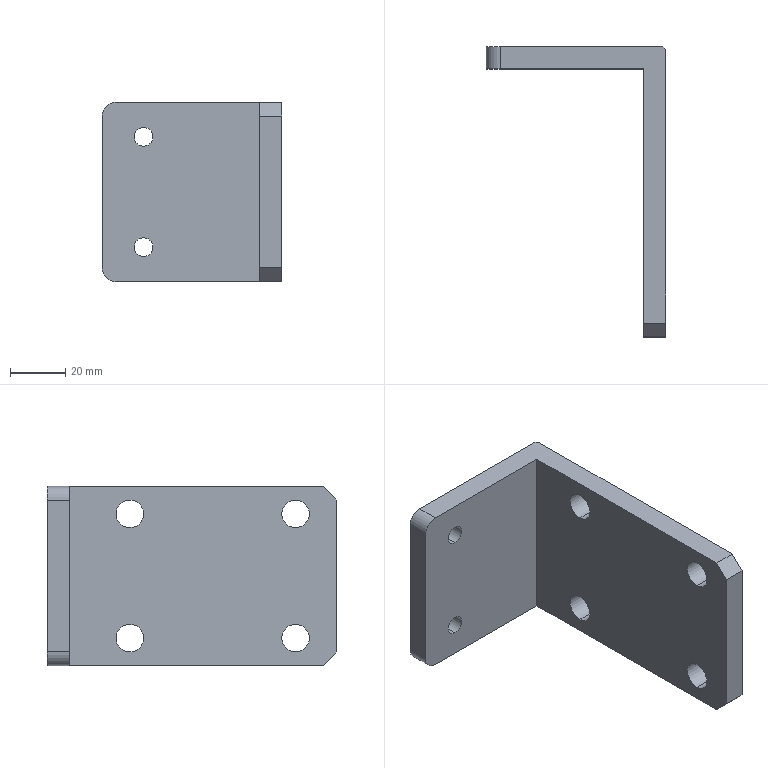Part | NX | features BREP 1 | 1 solid | 25 faces | box 65 x 105 x 65 mm | volume 80827 mm3 | cylinder 14 | plane 11 | commonest cylinder face diameters 10 x10 6.8 x4
STEP:
#1=CARTESIAN_POINT('',(0.,-30.,5.));
#2=VERTEX_POINT('',#1);
#3=CARTESIAN_POINT('',(0.,-30.,15.));
#4=VERTEX_POINT('',#3);
#5=CARTESIAN_POINT('',(0.,-30.,10.));
#6=DIRECTION('',(-1.,0.,0.));
#7=DIRECTION('',(0.,0.,1.));
#8=AXIS2_PLACEMENT_3D('',#5,#6,#7);
#9=CIRCLE('',#8,5.);
#10=EDGE_CURVE('',#2,#4,#9,.T.);
#11=ORIENTED_EDGE('',*,*,#10,.F.);
#12=CARTESIAN_POINT('',(-8.,-30.,5.));
#13=VERTEX_POINT('',#12);
#14=CARTESIAN_POINT('',(-8.,-30.,5.));
#15=DIRECTION('',(-1.,0.,0.));
#16=VECTOR('',#15,1000.);
#17=LINE('',#14,#16);
#18=EDGE_CURVE('',#13,#2,#17,.F.);
#19=ORIENTED_EDGE('',*,*,#18,.F.);
#20=CARTESIAN_POINT('',(-8.,-30.,15.));
#21=VERTEX_POINT('',#20);
#22=CARTESIAN_POINT('',(-8.,-30.,10.));
#23=DIRECTION('',(-1.,0.,0.));
#24=DIRECTION('',(0.,0.,1.));
#25=AXIS2_PLACEMENT_3D('',#22,#23,#24);
#26=CIRCLE('',#25,5.);
#27=EDGE_CURVE('',#13,#21,#26,.T.);
#28=ORIENTED_EDGE('',*,*,#27,.T.);
#29=CARTESIAN_POINT('',(-8.,-30.,15.));
#30=DIRECTION('',(-1.,0.,0.));
#31=VECTOR('',#30,1000.);
#32=LINE('',#29,#31);
#33=EDGE_CURVE('',#21,#4,#32,.F.);
#34=ORIENTED_EDGE('',*,*,#33,.T.);
#35=EDGE_LOOP('',(#11,#19,#28,#34));
#36=FACE_BOUND('',#35,.T.);
#37=CARTESIAN_POINT('',(-8.,-30.,10.));
#38=DIRECTION('',(-1.,0.,0.));
#39=DIRECTION('',(0.,0.,1.));
#40=AXIS2_PLACEMENT_3D('',#37,#38,#39);
#41=CYLINDRICAL_SURFACE('',#40,5.);
#42=ADVANCED_FACE('',(#36),#41,.F.);
#43=CARTESIAN_POINT('',(0.,-90.,50.));
#44=VERTEX_POINT('',#43);
#45=CARTESIAN_POINT('',(0.,-90.,60.));
#46=VERTEX_POINT('',#45);
#47=CARTESIAN_POINT('',(0.,-90.,55.));
#48=DIRECTION('',(-1.,0.,0.));
#49=DIRECTION('',(0.,0.,1.));
#50=AXIS2_PLACEMENT_3D('',#47,#48,#49);
#51=CIRCLE('',#50,5.);
#52=EDGE_CURVE('',#44,#46,#51,.T.);
#53=ORIENTED_EDGE('',*,*,#52,.F.);
#54=CARTESIAN_POINT('',(-8.,-90.,50.));
#55=VERTEX_POINT('',#54);
#56=CARTESIAN_POINT('',(-8.,-90.,50.));
#57=DIRECTION('',(-1.,0.,0.));
#58=VECTOR('',#57,1000.);
#59=LINE('',#56,#58);
#60=EDGE_CURVE('',#55,#44,#59,.F.);
#61=ORIENTED_EDGE('',*,*,#60,.F.);
#62=CARTESIAN_POINT('',(-8.,-90.,60.));
#63=VERTEX_POINT('',#62);
#64=CARTESIAN_POINT('',(-8.,-90.,55.));
#65=DIRECTION('',(-1.,0.,0.));
#66=DIRECTION('',(0.,0.,1.));
#67=AXIS2_PLACEMENT_3D('',#64,#65,#66);
#68=CIRCLE('',#67,5.);
#69=EDGE_CURVE('',#55,#63,#68,.T.);
#70=ORIENTED_EDGE('',*,*,#69,.T.);
#71=CARTESIAN_POINT('',(-8.,-90.,60.));
#72=DIRECTION('',(-1.,0.,0.));
#73=VECTOR('',#72,1000.);
#74=LINE('',#71,#73);
#75=EDGE_CURVE('',#63,#46,#74,.F.);
#76=ORIENTED_EDGE('',*,*,#75,.T.);
#77=EDGE_LOOP('',(#53,#61,#70,#76));
#78=FACE_BOUND('',#77,.T.);
#79=CARTESIAN_POINT('',(-8.,-90.,55.));
#80=DIRECTION('',(-1.,0.,0.));
#81=DIRECTION('',(0.,0.,1.));
#82=AXIS2_PLACEMENT_3D('',#79,#80,#81);
#83=CYLINDRICAL_SURFACE('',#82,5.);
#84=ADVANCED_FACE('',(#78),#83,.F.);
#85=CARTESIAN_POINT('',(0.,-90.,5.));
#86=VERTEX_POINT('',#85);
#87=CARTESIAN_POINT('',(0.,-90.,15.));
#88=VERTEX_POINT('',#87);
#89=CARTESIAN_POINT('',(0.,-90.,10.));
#90=DIRECTION('',(-1.,0.,0.));
#91=DIRECTION('',(0.,0.,1.));
#92=AXIS2_PLACEMENT_3D('',#89,#90,#91);
#93=CIRCLE('',#92,5.);
#94=EDGE_CURVE('',#86,#88,#93,.T.);
#95=ORIENTED_EDGE('',*,*,#94,.F.);
#96=CARTESIAN_POINT('',(-8.,-90.,5.));
#97=VERTEX_POINT('',#96);
#98=CARTESIAN_POINT('',(-8.,-90.,5.));
#99=DIRECTION('',(-1.,0.,0.));
#100=VECTOR('',#99,1000.);
#101=LINE('',#98,#100);
#102=EDGE_CURVE('',#97,#86,#101,.F.);
#103=ORIENTED_EDGE('',*,*,#102,.F.);
#104=CARTESIAN_POINT('',(-8.,-90.,15.));
#105=VERTEX_POINT('',#104);
#106=CARTESIAN_POINT('',(-8.,-90.,10.));
#107=DIRECTION('',(-1.,0.,0.));
#108=DIRECTION('',(0.,0.,1.));
#109=AXIS2_PLACEMENT_3D('',#106,#107,#108);
#110=CIRCLE('',#109,5.);
#111=EDGE_CURVE('',#97,#105,#110,.T.);
#112=ORIENTED_EDGE('',*,*,#111,.T.);
#113=CARTESIAN_POINT('',(-8.,-90.,15.));
#114=DIRECTION('',(-1.,0.,0.));
#115=VECTOR('',#114,1000.);
#116=LINE('',#113,#115);
#117=EDGE_CURVE('',#105,#88,#116,.F.);
#118=ORIENTED_EDGE('',*,*,#117,.T.);
#119=EDGE_LOOP('',(#95,#103,#112,#118));
#120=FACE_BOUND('',#119,.T.);
#121=CARTESIAN_POINT('',(-8.,-90.,10.));
#122=DIRECTION('',(-1.,0.,0.));
#123=DIRECTION('',(0.,0.,1.));
#124=AXIS2_PLACEMENT_3D('',#121,#122,#123);
#125=CYLINDRICAL_SURFACE('',#124,5.);
#126=ADVANCED_FACE('',(#120),#125,.F.);
#127=CARTESIAN_POINT('',(0.,-30.,50.));
#128=VERTEX_POINT('',#127);
#129=CARTESIAN_POINT('',(0.,-30.,60.));
#130=VERTEX_POINT('',#129);
#131=CARTESIAN_POINT('',(0.,-30.,55.));
#132=DIRECTION('',(-1.,0.,0.));
#133=DIRECTION('',(0.,0.,1.));
#134=AXIS2_PLACEMENT_3D('',#131,#132,#133);
#135=CIRCLE('',#134,5.);
#136=EDGE_CURVE('',#128,#130,#135,.T.);
#137=ORIENTED_EDGE('',*,*,#136,.F.);
#138=CARTESIAN_POINT('',(-8.,-30.,50.));
#139=VERTEX_POINT('',#138);
#140=CARTESIAN_POINT('',(-8.,-30.,50.));
#141=DIRECTION('',(-1.,0.,0.));
#142=VECTOR('',#141,1000.);
#143=LINE('',#140,#142);
#144=EDGE_CURVE('',#139,#128,#143,.F.);
#145=ORIENTED_EDGE('',*,*,#144,.F.);
#146=CARTESIAN_POINT('',(-8.,-30.,60.));
#147=VERTEX_POINT('',#146);
#148=CARTESIAN_POINT('',(-8.,-30.,55.));
#149=DIRECTION('',(-1.,0.,0.));
#150=DIRECTION('',(0.,0.,1.));
#151=AXIS2_PLACEMENT_3D('',#148,#149,#150);
#152=CIRCLE('',#151,5.);
#153=EDGE_CURVE('',#139,#147,#152,.T.);
#154=ORIENTED_EDGE('',*,*,#153,.T.);
#155=CARTESIAN_POINT('',(-8.,-30.,60.));
#156=DIRECTION('',(-1.,0.,0.));
#157=VECTOR('',#156,1000.);
#158=LINE('',#155,#157);
#159=EDGE_CURVE('',#147,#130,#158,.F.);
#160=ORIENTED_EDGE('',*,*,#159,.T.);
#161=EDGE_LOOP('',(#137,#145,#154,#160));
#162=FACE_BOUND('',#161,.T.);
#163=CARTESIAN_POINT('',(-8.,-30.,55.));
#164=DIRECTION('',(-1.,0.,0.));
#165=DIRECTION('',(0.,0.,1.));
#166=AXIS2_PLACEMENT_3D('',#163,#164,#165);
#167=CYLINDRICAL_SURFACE('',#166,5.);
#168=ADVANCED_FACE('',(#162),#167,.F.);
#169=CARTESIAN_POINT('',(-50.,-8.,9.1));
#170=VERTEX_POINT('',#169);
#171=CARTESIAN_POINT('',(-50.,-8.,15.9));
#172=VERTEX_POINT('',#171);
#173=CARTESIAN_POINT('',(-50.,-8.,12.5));
#174=DIRECTION('',(0.,1.,0.));
#175=DIRECTION('',(-1.,0.,0.));
#176=AXIS2_PLACEMENT_3D('',#173,#174,#175);
#177=CIRCLE('',#176,3.4);
#178=EDGE_CURVE('',#170,#172,#177,.T.);
#179=ORIENTED_EDGE('',*,*,#178,.F.);
#180=CARTESIAN_POINT('',(-50.,0.,9.1));
#181=VERTEX_POINT('',#180);
#182=CARTESIAN_POINT('',(-50.,0.,9.1));
#183=DIRECTION('',(0.,1.,0.));
#184=VECTOR('',#183,1000.);
#185=LINE('',#182,#184);
#186=EDGE_CURVE('',#181,#170,#185,.F.);
#187=ORIENTED_EDGE('',*,*,#186,.F.);
#188=CARTESIAN_POINT('',(-50.,0.,15.9));
#189=VERTEX_POINT('',#188);
#190=CARTESIAN_POINT('',(-50.,0.,12.5));
#191=DIRECTION('',(0.,1.,0.));
#192=DIRECTION('',(0.,0.,1.));
#193=AXIS2_PLACEMENT_3D('',#190,#191,#192);
#194=CIRCLE('',#193,3.4);
#195=EDGE_CURVE('',#181,#189,#194,.T.);
#196=ORIENTED_EDGE('',*,*,#195,.T.);
#197=CARTESIAN_POINT('',(-50.,0.,15.9));
#198=DIRECTION('',(0.,1.,0.));
#199=VECTOR('',#198,1000.);
#200=LINE('',#197,#199);
#201=EDGE_CURVE('',#189,#172,#200,.F.);
#202=ORIENTED_EDGE('',*,*,#201,.T.);
#203=EDGE_LOOP('',(#179,#187,#196,#202));
#204=FACE_BOUND('',#203,.T.);
#205=CARTESIAN_POINT('',(-50.,0.,12.5));
#206=DIRECTION('',(0.,1.,0.));
#207=DIRECTION('',(0.,0.,1.));
#208=AXIS2_PLACEMENT_3D('',#205,#206,#207);
#209=CYLINDRICAL_SURFACE('',#208,3.4);
#210=ADVANCED_FACE('',(#204),#209,.F.);
#211=CARTESIAN_POINT('',(-50.,-8.,49.1));
#212=VERTEX_POINT('',#211);
#213=CARTESIAN_POINT('',(-50.,-8.,55.9));
#214=VERTEX_POINT('',#213);
#215=CARTESIAN_POINT('',(-50.,-8.,52.5));
#216=DIRECTION('',(0.,1.,0.));
#217=DIRECTION('',(-1.,0.,0.));
#218=AXIS2_PLACEMENT_3D('',#215,#216,#217);
#219=CIRCLE('',#218,3.4);
#220=EDGE_CURVE('',#212,#214,#219,.T.);
#221=ORIENTED_EDGE('',*,*,#220,.F.);
#222=CARTESIAN_POINT('',(-50.,0.,49.1));
#223=VERTEX_POINT('',#222);
#224=CARTESIAN_POINT('',(-50.,0.,49.1));
#225=DIRECTION('',(0.,1.,0.));
#226=VECTOR('',#225,1000.);
#227=LINE('',#224,#226);
#228=EDGE_CURVE('',#223,#212,#227,.F.);
#229=ORIENTED_EDGE('',*,*,#228,.F.);
#230=CARTESIAN_POINT('',(-50.,0.,55.9));
#231=VERTEX_POINT('',#230);
#232=CARTESIAN_POINT('',(-50.,0.,52.5));
#233=DIRECTION('',(0.,1.,0.));
#234=DIRECTION('',(0.,0.,1.));
#235=AXIS2_PLACEMENT_3D('',#232,#233,#234);
#236=CIRCLE('',#235,3.4);
#237=EDGE_CURVE('',#223,#231,#236,.T.);
#238=ORIENTED_EDGE('',*,*,#237,.T.);
#239=CARTESIAN_POINT('',(-50.,0.,55.9));
#240=DIRECTION('',(0.,1.,0.));
#241=VECTOR('',#240,1000.);
#242=LINE('',#239,#241);
#243=EDGE_CURVE('',#231,#214,#242,.F.);
#244=ORIENTED_EDGE('',*,*,#243,.T.);
#245=EDGE_LOOP('',(#221,#229,#238,#244));
#246=FACE_BOUND('',#245,.T.);
#247=CARTESIAN_POINT('',(-50.,0.,52.5));
#248=DIRECTION('',(0.,1.,0.));
#249=DIRECTION('',(0.,0.,1.));
#250=AXIS2_PLACEMENT_3D('',#247,#248,#249);
#251=CYLINDRICAL_SURFACE('',#250,3.4);
#252=ADVANCED_FACE('',(#246),#251,.F.);
#253=CARTESIAN_POINT('',(-8.,-105.,60.));
#254=VERTEX_POINT('',#253);
#255=CARTESIAN_POINT('',(-8.,-105.,5.));
#256=VERTEX_POINT('',#255);
#257=CARTESIAN_POINT('',(-8.,-105.,65.));
#258=DIRECTION('',(0.,0.,-1.));
#259=VECTOR('',#258,1000.);
#260=LINE('',#257,#259);
#261=EDGE_CURVE('',#254,#256,#260,.T.);
#262=ORIENTED_EDGE('',*,*,#261,.F.);
#263=CARTESIAN_POINT('',(-8.,-100.,65.));
#264=VERTEX_POINT('',#263);
#265=CARTESIAN_POINT('',(-8.,-100.,65.));
#266=DIRECTION('',(0.,0.7071,0.7071));
#267=VECTOR('',#266,1000.);
#268=LINE('',#265,#267);
#269=EDGE_CURVE('',#254,#264,#268,.T.);
#270=ORIENTED_EDGE('',*,*,#269,.T.);
#271=CARTESIAN_POINT('',(-8.,-8.,65.));
#272=VERTEX_POINT('',#271);
#273=CARTESIAN_POINT('',(-8.,-8.,65.));
#274=DIRECTION('',(0.,-1.,0.));
#275=VECTOR('',#274,1000.);
#276=LINE('',#273,#275);
#277=EDGE_CURVE('',#272,#264,#276,.T.);
#278=ORIENTED_EDGE('',*,*,#277,.F.);
#279=CARTESIAN_POINT('',(-8.,-8.,0.));
#280=VERTEX_POINT('',#279);
#281=CARTESIAN_POINT('',(-8.,-8.,65.));
#282=DIRECTION('',(0.,0.,-1.));
#283=VECTOR('',#282,1000.);
#284=LINE('',#281,#283);
#285=EDGE_CURVE('',#272,#280,#284,.T.);
#286=ORIENTED_EDGE('',*,*,#285,.T.);
#287=CARTESIAN_POINT('',(-8.,-100.,0.));
#288=VERTEX_POINT('',#287);
#289=CARTESIAN_POINT('',(-8.,-8.,0.));
#290=DIRECTION('',(0.,-1.,0.));
#291=VECTOR('',#290,1000.);
#292=LINE('',#289,#291);
#293=EDGE_CURVE('',#280,#288,#292,.T.);
#294=ORIENTED_EDGE('',*,*,#293,.T.);
#295=CARTESIAN_POINT('',(-8.,-105.,5.));
#296=DIRECTION('',(0.,-0.7071,0.7071));
#297=VECTOR('',#296,1000.);
#298=LINE('',#295,#297);
#299=EDGE_CURVE('',#288,#256,#298,.T.);
#300=ORIENTED_EDGE('',*,*,#299,.T.);
#301=EDGE_LOOP('',(#262,#270,#278,#286,#294,#300));
#302=FACE_BOUND('',#301,.T.);
#303=CARTESIAN_POINT('',(-8.,-90.,55.));
#304=DIRECTION('',(-1.,0.,0.));
#305=DIRECTION('',(0.,0.,1.));
#306=AXIS2_PLACEMENT_3D('',#303,#304,#305);
#307=CIRCLE('',#306,5.);
#308=EDGE_CURVE('',#63,#55,#307,.T.);
#309=ORIENTED_EDGE('',*,*,#308,.F.);
#310=ORIENTED_EDGE('',*,*,#69,.F.);
#311=EDGE_LOOP('',(#309,#310));
#312=FACE_BOUND('',#311,.T.);
#313=CARTESIAN_POINT('',(-8.,-90.,10.));
#314=DIRECTION('',(-1.,0.,0.));
#315=DIRECTION('',(0.,0.,1.));
#316=AXIS2_PLACEMENT_3D('',#313,#314,#315);
#317=CIRCLE('',#316,5.);
#318=EDGE_CURVE('',#105,#97,#317,.T.);
#319=ORIENTED_EDGE('',*,*,#318,.F.);
#320=ORIENTED_EDGE('',*,*,#111,.F.);
#321=EDGE_LOOP('',(#319,#320));
#322=FACE_BOUND('',#321,.T.);
#323=CARTESIAN_POINT('',(-8.,-30.,55.));
#324=DIRECTION('',(-1.,0.,0.));
#325=DIRECTION('',(0.,0.,1.));
#326=AXIS2_PLACEMENT_3D('',#323,#324,#325);
#327=CIRCLE('',#326,5.);
#328=EDGE_CURVE('',#147,#139,#327,.T.);
#329=ORIENTED_EDGE('',*,*,#328,.F.);
#330=ORIENTED_EDGE('',*,*,#153,.F.);
#331=EDGE_LOOP('',(#329,#330));
#332=FACE_BOUND('',#331,.T.);
#333=CARTESIAN_POINT('',(-8.,-30.,10.));
#334=DIRECTION('',(-1.,0.,0.));
#335=DIRECTION('',(0.,0.,1.));
#336=AXIS2_PLACEMENT_3D('',#333,#334,#335);
#337=CIRCLE('',#336,5.);
#338=EDGE_CURVE('',#21,#13,#337,.T.);
#339=ORIENTED_EDGE('',*,*,#338,.F.);
#340=ORIENTED_EDGE('',*,*,#27,.F.);
#341=EDGE_LOOP('',(#339,#340));
#342=FACE_BOUND('',#341,.T.);
#343=CARTESIAN_POINT('',(-8.,-8.,65.));
#344=DIRECTION('',(1.,0.,0.));
#345=DIRECTION('',(0.,1.,0.));
#346=AXIS2_PLACEMENT_3D('',#343,#344,#345);
#347=PLANE('',#346);
#348=ADVANCED_FACE('',(#302,#312,#322,#332,#342),#347,.F.);
#349=CARTESIAN_POINT('',(0.,-100.,0.));
#350=VERTEX_POINT('',#349);
#351=CARTESIAN_POINT('',(0.,-1.,0.));
#352=VERTEX_POINT('',#351);
#353=CARTESIAN_POINT('',(0.,-105.,0.));
#354=DIRECTION('',(0.,1.,0.));
#355=VECTOR('',#354,1000.);
#356=LINE('',#353,#355);
#357=EDGE_CURVE('',#350,#352,#356,.T.);
#358=ORIENTED_EDGE('',*,*,#357,.T.);
#359=CARTESIAN_POINT('',(0.,-1.,65.));
#360=VERTEX_POINT('',#359);
#361=CARTESIAN_POINT('',(0.,-1.,65.));
#362=DIRECTION('',(0.,0.,1.));
#363=VECTOR('',#362,1000.);
#364=LINE('',#361,#363);
#365=EDGE_CURVE('',#352,#360,#364,.T.);
#366=ORIENTED_EDGE('',*,*,#365,.T.);
#367=CARTESIAN_POINT('',(0.,-100.,65.));
#368=VERTEX_POINT('',#367);
#369=CARTESIAN_POINT('',(0.,-105.,65.));
#370=DIRECTION('',(0.,1.,0.));
#371=VECTOR('',#370,1000.);
#372=LINE('',#369,#371);
#373=EDGE_CURVE('',#368,#360,#372,.T.);
#374=ORIENTED_EDGE('',*,*,#373,.F.);
#375=CARTESIAN_POINT('',(0.,-105.,60.));
#376=VERTEX_POINT('',#375);
#377=CARTESIAN_POINT('',(0.,-100.,65.));
#378=DIRECTION('',(0.,-0.7071,-0.7071));
#379=VECTOR('',#378,1000.);
#380=LINE('',#377,#379);
#381=EDGE_CURVE('',#368,#376,#380,.T.);
#382=ORIENTED_EDGE('',*,*,#381,.T.);
#383=CARTESIAN_POINT('',(0.,-105.,5.));
#384=VERTEX_POINT('',#383);
#385=CARTESIAN_POINT('',(0.,-105.,65.));
#386=DIRECTION('',(0.,0.,-1.));
#387=VECTOR('',#386,1000.);
#388=LINE('',#385,#387);
#389=EDGE_CURVE('',#376,#384,#388,.T.);
#390=ORIENTED_EDGE('',*,*,#389,.T.);
#391=CARTESIAN_POINT('',(0.,-105.,5.));
#392=DIRECTION('',(0.,0.7071,-0.7071));
#393=VECTOR('',#392,1000.);
#394=LINE('',#391,#393);
#395=EDGE_CURVE('',#384,#350,#394,.T.);
#396=ORIENTED_EDGE('',*,*,#395,.T.);
#397=EDGE_LOOP('',(#358,#366,#374,#382,#390,#396));
#398=FACE_BOUND('',#397,.T.);
#399=CARTESIAN_POINT('',(0.,-30.,10.));
#400=DIRECTION('',(-1.,0.,0.));
#401=DIRECTION('',(0.,0.,1.));
#402=AXIS2_PLACEMENT_3D('',#399,#400,#401);
#403=CIRCLE('',#402,5.);
#404=EDGE_CURVE('',#4,#2,#403,.T.);
#405=ORIENTED_EDGE('',*,*,#404,.T.);
#406=ORIENTED_EDGE('',*,*,#10,.T.);
#407=EDGE_LOOP('',(#405,#406));
#408=FACE_BOUND('',#407,.T.);
#409=CARTESIAN_POINT('',(0.,-90.,55.));
#410=DIRECTION('',(-1.,0.,0.));
#411=DIRECTION('',(0.,0.,1.));
#412=AXIS2_PLACEMENT_3D('',#409,#410,#411);
#413=CIRCLE('',#412,5.);
#414=EDGE_CURVE('',#46,#44,#413,.T.);
#415=ORIENTED_EDGE('',*,*,#414,.T.);
#416=ORIENTED_EDGE('',*,*,#52,.T.);
#417=EDGE_LOOP('',(#415,#416));
#418=FACE_BOUND('',#417,.T.);
#419=CARTESIAN_POINT('',(0.,-90.,10.));
#420=DIRECTION('',(-1.,0.,0.));
#421=DIRECTION('',(0.,0.,1.));
#422=AXIS2_PLACEMENT_3D('',#419,#420,#421);
#423=CIRCLE('',#422,5.);
#424=EDGE_CURVE('',#88,#86,#423,.T.);
#425=ORIENTED_EDGE('',*,*,#424,.T.);
#426=ORIENTED_EDGE('',*,*,#94,.T.);
#427=EDGE_LOOP('',(#425,#426));
#428=FACE_BOUND('',#427,.T.);
#429=CARTESIAN_POINT('',(0.,-30.,55.));
#430=DIRECTION('',(-1.,0.,0.));
#431=DIRECTION('',(0.,0.,1.));
#432=AXIS2_PLACEMENT_3D('',#429,#430,#431);
#433=CIRCLE('',#432,5.);
#434=EDGE_CURVE('',#130,#128,#433,.T.);
#435=ORIENTED_EDGE('',*,*,#434,.T.);
#436=ORIENTED_EDGE('',*,*,#136,.T.);
#437=EDGE_LOOP('',(#435,#436));
#438=FACE_BOUND('',#437,.T.);
#439=CARTESIAN_POINT('',(0.,-105.,65.));
#440=DIRECTION('',(-1.,0.,0.));
#441=DIRECTION('',(0.,1.,0.));
#442=AXIS2_PLACEMENT_3D('',#439,#440,#441);
#443=PLANE('',#442);
#444=ADVANCED_FACE('',(#398,#408,#418,#428,#438),#443,.F.);
#445=CARTESIAN_POINT('',(-1.,0.,65.));
#446=VERTEX_POINT('',#445);
#447=CARTESIAN_POINT('',(-60.,0.,65.));
#448=VERTEX_POINT('',#447);
#449=CARTESIAN_POINT('',(0.,0.,65.));
#450=DIRECTION('',(-1.,0.,0.));
#451=VECTOR('',#450,1000.);
#452=LINE('',#449,#451);
#453=EDGE_CURVE('',#446,#448,#452,.T.);
#454=ORIENTED_EDGE('',*,*,#453,.F.);
#455=CARTESIAN_POINT('',(-1.,0.,0.));
#456=VERTEX_POINT('',#455);
#457=CARTESIAN_POINT('',(-1.,0.,65.));
#458=DIRECTION('',(0.,0.,-1.));
#459=VECTOR('',#458,1000.);
#460=LINE('',#457,#459);
#461=EDGE_CURVE('',#446,#456,#460,.T.);
#462=ORIENTED_EDGE('',*,*,#461,.T.);
#463=CARTESIAN_POINT('',(-60.,0.,0.));
#464=VERTEX_POINT('',#463);
#465=CARTESIAN_POINT('',(0.,0.,0.));
#466=DIRECTION('',(-1.,0.,0.));
#467=VECTOR('',#466,1000.);
#468=LINE('',#465,#467);
#469=EDGE_CURVE('',#456,#464,#468,.T.);
#470=ORIENTED_EDGE('',*,*,#469,.T.);
#471=CARTESIAN_POINT('',(-65.,0.,5.));
#472=VERTEX_POINT('',#471);
#473=CARTESIAN_POINT('',(-60.,0.,5.));
#474=DIRECTION('',(0.,1.,0.));
#475=DIRECTION('',(1.,0.,0.));
#476=AXIS2_PLACEMENT_3D('',#473,#474,#475);
#477=CIRCLE('',#476,5.);
#478=EDGE_CURVE('',#464,#472,#477,.T.);
#479=ORIENTED_EDGE('',*,*,#478,.T.);
#480=CARTESIAN_POINT('',(-65.,0.,60.));
#481=VERTEX_POINT('',#480);
#482=CARTESIAN_POINT('',(-65.,0.,65.));
#483=DIRECTION('',(0.,0.,-1.));
#484=VECTOR('',#483,1000.);
#485=LINE('',#482,#484);
#486=EDGE_CURVE('',#481,#472,#485,.T.);
#487=ORIENTED_EDGE('',*,*,#486,.F.);
#488=CARTESIAN_POINT('',(-60.,0.,60.));
#489=DIRECTION('',(0.,1.,0.));
#490=DIRECTION('',(1.,0.,0.));
#491=AXIS2_PLACEMENT_3D('',#488,#489,#490);
#492=CIRCLE('',#491,5.);
#493=EDGE_CURVE('',#481,#448,#492,.T.);
#494=ORIENTED_EDGE('',*,*,#493,.T.);
#495=EDGE_LOOP('',(#454,#462,#470,#479,#487,#494));
#496=FACE_BOUND('',#495,.T.);
#497=CARTESIAN_POINT('',(-50.,0.,12.5));
#498=DIRECTION('',(0.,1.,0.));
#499=DIRECTION('',(0.,0.,1.));
#500=AXIS2_PLACEMENT_3D('',#497,#498,#499);
#501=CIRCLE('',#500,3.4);
#502=EDGE_CURVE('',#189,#181,#501,.T.);
#503=ORIENTED_EDGE('',*,*,#502,.F.);
#504=ORIENTED_EDGE('',*,*,#195,.F.);
#505=EDGE_LOOP('',(#503,#504));
#506=FACE_BOUND('',#505,.T.);
#507=CARTESIAN_POINT('',(-50.,0.,52.5));
#508=DIRECTION('',(0.,1.,0.));
#509=DIRECTION('',(0.,0.,1.));
#510=AXIS2_PLACEMENT_3D('',#507,#508,#509);
#511=CIRCLE('',#510,3.4);
#512=EDGE_CURVE('',#231,#223,#511,.T.);
#513=ORIENTED_EDGE('',*,*,#512,.F.);
#514=ORIENTED_EDGE('',*,*,#237,.F.);
#515=EDGE_LOOP('',(#513,#514));
#516=FACE_BOUND('',#515,.T.);
#517=CARTESIAN_POINT('',(0.,0.,65.));
#518=DIRECTION('',(0.,-1.,0.));
#519=DIRECTION('',(0.,0.,-1.));
#520=AXIS2_PLACEMENT_3D('',#517,#518,#519);
#521=PLANE('',#520);
#522=ADVANCED_FACE('',(#496,#506,#516),#521,.F.);
#523=ORIENTED_EDGE('',*,*,#486,.T.);
#524=CARTESIAN_POINT('',(-65.,-8.,5.));
#525=VERTEX_POINT('',#524);
#526=CARTESIAN_POINT('',(-65.,0.,5.));
#527=DIRECTION('',(0.,-1.,0.));
#528=VECTOR('',#527,1000.);
#529=LINE('',#526,#528);
#530=EDGE_CURVE('',#472,#525,#529,.T.);
#531=ORIENTED_EDGE('',*,*,#530,.T.);
#532=CARTESIAN_POINT('',(-65.,-8.,60.));
#533=VERTEX_POINT('',#532);
#534=CARTESIAN_POINT('',(-65.,-8.,65.));
#535=DIRECTION('',(0.,0.,-1.));
#536=VECTOR('',#535,1000.);
#537=LINE('',#534,#536);
#538=EDGE_CURVE('',#533,#525,#537,.T.);
#539=ORIENTED_EDGE('',*,*,#538,.F.);
#540=CARTESIAN_POINT('',(-65.,0.,60.));
#541=DIRECTION('',(0.,1.,0.));
#542=VECTOR('',#541,1000.);
#543=LINE('',#540,#542);
#544=EDGE_CURVE('',#533,#481,#543,.T.);
#545=ORIENTED_EDGE('',*,*,#544,.T.);
#546=EDGE_LOOP('',(#523,#531,#539,#545));
#547=FACE_BOUND('',#546,.T.);
#548=CARTESIAN_POINT('',(-65.,0.,65.));
#549=DIRECTION('',(1.,0.,0.));
#550=DIRECTION('',(0.,1.,0.));
#551=AXIS2_PLACEMENT_3D('',#548,#549,#550);
#552=PLANE('',#551);
#553=ADVANCED_FACE('',(#547),#552,.F.);
#554=ORIENTED_EDGE('',*,*,#538,.T.);
#555=CARTESIAN_POINT('',(-60.,-8.,0.));
#556=VERTEX_POINT('',#555);
#557=CARTESIAN_POINT('',(-60.,-8.,5.));
#558=DIRECTION('',(0.,-1.,0.));
#559=DIRECTION('',(-1.,0.,0.));
#560=AXIS2_PLACEMENT_3D('',#557,#558,#559);
#561=CIRCLE('',#560,5.);
#562=EDGE_CURVE('',#525,#556,#561,.T.);
#563=ORIENTED_EDGE('',*,*,#562,.T.);
#564=CARTESIAN_POINT('',(-65.,-8.,0.));
#565=DIRECTION('',(1.,0.,0.));
#566=VECTOR('',#565,1000.);
#567=LINE('',#564,#566);
#568=EDGE_CURVE('',#556,#280,#567,.T.);
#569=ORIENTED_EDGE('',*,*,#568,.T.);
#570=ORIENTED_EDGE('',*,*,#285,.F.);
#571=CARTESIAN_POINT('',(-60.,-8.,65.));
#572=VERTEX_POINT('',#571);
#573=CARTESIAN_POINT('',(-65.,-8.,65.));
#574=DIRECTION('',(1.,0.,0.));
#575=VECTOR('',#574,1000.);
#576=LINE('',#573,#575);
#577=EDGE_CURVE('',#572,#272,#576,.T.);
#578=ORIENTED_EDGE('',*,*,#577,.F.);
#579=CARTESIAN_POINT('',(-60.,-8.,60.));
#580=DIRECTION('',(0.,-1.,0.));
#581=DIRECTION('',(-1.,0.,0.));
#582=AXIS2_PLACEMENT_3D('',#579,#580,#581);
#583=CIRCLE('',#582,5.);
#584=EDGE_CURVE('',#572,#533,#583,.T.);
#585=ORIENTED_EDGE('',*,*,#584,.T.);
#586=EDGE_LOOP('',(#554,#563,#569,#570,#578,#585));
#587=FACE_BOUND('',#586,.T.);
#588=CARTESIAN_POINT('',(-50.,-8.,12.5));
#589=DIRECTION('',(0.,1.,0.));
#590=DIRECTION('',(-1.,0.,0.));
#591=AXIS2_PLACEMENT_3D('',#588,#589,#590);
#592=CIRCLE('',#591,3.4);
#593=EDGE_CURVE('',#172,#170,#592,.T.);
#594=ORIENTED_EDGE('',*,*,#593,.T.);
#595=ORIENTED_EDGE('',*,*,#178,.T.);
#596=EDGE_LOOP('',(#594,#595));
#597=FACE_BOUND('',#596,.T.);
#598=CARTESIAN_POINT('',(-50.,-8.,52.5));
#599=DIRECTION('',(0.,1.,0.));
#600=DIRECTION('',(-1.,0.,0.));
#601=AXIS2_PLACEMENT_3D('',#598,#599,#600);
#602=CIRCLE('',#601,3.4);
#603=EDGE_CURVE('',#214,#212,#602,.T.);
#604=ORIENTED_EDGE('',*,*,#603,.T.);
#605=ORIENTED_EDGE('',*,*,#220,.T.);
#606=EDGE_LOOP('',(#604,#605));
#607=FACE_BOUND('',#606,.T.);
#608=CARTESIAN_POINT('',(-65.,-8.,65.));
#609=DIRECTION('',(0.,1.,0.));
#610=DIRECTION('',(1.,0.,0.));
#611=AXIS2_PLACEMENT_3D('',#608,#609,#610);
#612=PLANE('',#611);
#613=ADVANCED_FACE('',(#587,#597,#607),#612,.F.);
#614=ORIENTED_EDGE('',*,*,#389,.F.);
#615=CARTESIAN_POINT('',(-8.,-105.,60.));
#616=DIRECTION('',(-1.,0.,0.));
#617=VECTOR('',#616,1000.);
#618=LINE('',#615,#617);
#619=EDGE_CURVE('',#376,#254,#618,.T.);
#620=ORIENTED_EDGE('',*,*,#619,.T.);
#621=ORIENTED_EDGE('',*,*,#261,.T.);
#622=CARTESIAN_POINT('',(-8.,-105.,5.));
#623=DIRECTION('',(1.,0.,0.));
#624=VECTOR('',#623,1000.);
#625=LINE('',#622,#624);
#626=EDGE_CURVE('',#256,#384,#625,.T.);
#627=ORIENTED_EDGE('',*,*,#626,.T.);
#628=EDGE_LOOP('',(#614,#620,#621,#627));
#629=FACE_BOUND('',#628,.T.);
#630=CARTESIAN_POINT('',(-8.,-105.,65.));
#631=DIRECTION('',(0.,1.,0.));
#632=DIRECTION('',(1.,0.,0.));
#633=AXIS2_PLACEMENT_3D('',#630,#631,#632);
#634=PLANE('',#633);
#635=ADVANCED_FACE('',(#629),#634,.F.);
#636=ORIENTED_EDGE('',*,*,#373,.T.);
#637=CARTESIAN_POINT('',(-0.5,-0.5,65.));
#638=DIRECTION('',(-0.7071,0.7071,0.));
#639=VECTOR('',#638,1000.);
#640=LINE('',#637,#639);
#641=EDGE_CURVE('',#360,#446,#640,.T.);
#642=ORIENTED_EDGE('',*,*,#641,.T.);
#643=ORIENTED_EDGE('',*,*,#453,.T.);
#644=CARTESIAN_POINT('',(-60.,-8.,65.));
#645=DIRECTION('',(0.,-1.,0.));
#646=VECTOR('',#645,1000.);
#647=LINE('',#644,#646);
#648=EDGE_CURVE('',#448,#572,#647,.T.);
#649=ORIENTED_EDGE('',*,*,#648,.T.);
#650=ORIENTED_EDGE('',*,*,#577,.T.);
#651=ORIENTED_EDGE('',*,*,#277,.T.);
#652=CARTESIAN_POINT('',(0.,-100.,65.));
#653=DIRECTION('',(1.,0.,0.));
#654=VECTOR('',#653,1000.);
#655=LINE('',#652,#654);
#656=EDGE_CURVE('',#264,#368,#655,.T.);
#657=ORIENTED_EDGE('',*,*,#656,.T.);
#658=EDGE_LOOP('',(#636,#642,#643,#649,#650,#651,#657));
#659=FACE_BOUND('',#658,.T.);
#660=CARTESIAN_POINT('',(0.,0.,65.));
#661=DIRECTION('',(0.,0.,1.));
#662=DIRECTION('',(1.,0.,0.));
#663=AXIS2_PLACEMENT_3D('',#660,#661,#662);
#664=PLANE('',#663);
#665=ADVANCED_FACE('',(#659),#664,.T.);
#666=ORIENTED_EDGE('',*,*,#469,.F.);
#667=CARTESIAN_POINT('',(-1.,0.,0.));
#668=DIRECTION('',(0.7071,-0.7071,0.));
#669=VECTOR('',#668,1000.);
#670=LINE('',#667,#669);
#671=EDGE_CURVE('',#456,#352,#670,.T.);
#672=ORIENTED_EDGE('',*,*,#671,.T.);
#673=ORIENTED_EDGE('',*,*,#357,.F.);
#674=CARTESIAN_POINT('',(0.,-100.,0.));
#675=DIRECTION('',(-1.,0.,0.));
#676=VECTOR('',#675,1000.);
#677=LINE('',#674,#676);
#678=EDGE_CURVE('',#350,#288,#677,.T.);
#679=ORIENTED_EDGE('',*,*,#678,.T.);
#680=ORIENTED_EDGE('',*,*,#293,.F.);
#681=ORIENTED_EDGE('',*,*,#568,.F.);
#682=CARTESIAN_POINT('',(-60.,0.,0.));
#683=DIRECTION('',(0.,1.,0.));
#684=VECTOR('',#683,1000.);
#685=LINE('',#682,#684);
#686=EDGE_CURVE('',#556,#464,#685,.T.);
#687=ORIENTED_EDGE('',*,*,#686,.T.);
#688=EDGE_LOOP('',(#666,#672,#673,#679,#680,#681,#687));
#689=FACE_BOUND('',#688,.T.);
#690=CARTESIAN_POINT('',(0.,0.,0.));
#691=DIRECTION('',(0.,0.,1.));
#692=DIRECTION('',(1.,0.,0.));
#693=AXIS2_PLACEMENT_3D('',#690,#691,#692);
#694=PLANE('',#693);
#695=ADVANCED_FACE('',(#689),#694,.F.);
#696=ORIENTED_EDGE('',*,*,#478,.F.);
#697=ORIENTED_EDGE('',*,*,#686,.F.);
#698=ORIENTED_EDGE('',*,*,#562,.F.);
#699=ORIENTED_EDGE('',*,*,#530,.F.);
#700=EDGE_LOOP('',(#696,#697,#698,#699));
#701=FACE_BOUND('',#700,.T.);
#702=CARTESIAN_POINT('',(-60.,0.,5.));
#703=DIRECTION('',(0.,-1.,0.));
#704=DIRECTION('',(0.,0.,-1.));
#705=AXIS2_PLACEMENT_3D('',#702,#703,#704);
#706=CYLINDRICAL_SURFACE('',#705,5.);
#707=ADVANCED_FACE('',(#701),#706,.T.);
#708=ORIENTED_EDGE('',*,*,#493,.F.);
#709=ORIENTED_EDGE('',*,*,#544,.F.);
#710=ORIENTED_EDGE('',*,*,#584,.F.);
#711=ORIENTED_EDGE('',*,*,#648,.F.);
#712=EDGE_LOOP('',(#708,#709,#710,#711));
#713=FACE_BOUND('',#712,.T.);
#714=CARTESIAN_POINT('',(-60.,0.,60.));
#715=DIRECTION('',(0.,1.,0.));
#716=DIRECTION('',(0.,0.,1.));
#717=AXIS2_PLACEMENT_3D('',#714,#715,#716);
#718=CYLINDRICAL_SURFACE('',#717,5.);
#719=ADVANCED_FACE('',(#713),#718,.T.);
#720=ORIENTED_EDGE('',*,*,#228,.T.);
#721=ORIENTED_EDGE('',*,*,#603,.F.);
#722=ORIENTED_EDGE('',*,*,#243,.F.);
#723=ORIENTED_EDGE('',*,*,#512,.T.);
#724=EDGE_LOOP('',(#720,#721,#722,#723));
#725=FACE_BOUND('',#724,.T.);
#726=CARTESIAN_POINT('',(-50.,0.,52.5));
#727=DIRECTION('',(0.,1.,0.));
#728=DIRECTION('',(0.,0.,1.));
#729=AXIS2_PLACEMENT_3D('',#726,#727,#728);
#730=CYLINDRICAL_SURFACE('',#729,3.4);
#731=ADVANCED_FACE('',(#725),#730,.F.);
#732=ORIENTED_EDGE('',*,*,#186,.T.);
#733=ORIENTED_EDGE('',*,*,#593,.F.);
#734=ORIENTED_EDGE('',*,*,#201,.F.);
#735=ORIENTED_EDGE('',*,*,#502,.T.);
#736=EDGE_LOOP('',(#732,#733,#734,#735));
#737=FACE_BOUND('',#736,.T.);
#738=CARTESIAN_POINT('',(-50.,0.,12.5));
#739=DIRECTION('',(0.,1.,0.));
#740=DIRECTION('',(0.,0.,1.));
#741=AXIS2_PLACEMENT_3D('',#738,#739,#740);
#742=CYLINDRICAL_SURFACE('',#741,3.4);
#743=ADVANCED_FACE('',(#737),#742,.F.);
#744=ORIENTED_EDGE('',*,*,#144,.T.);
#745=ORIENTED_EDGE('',*,*,#434,.F.);
#746=ORIENTED_EDGE('',*,*,#159,.F.);
#747=ORIENTED_EDGE('',*,*,#328,.T.);
#748=EDGE_LOOP('',(#744,#745,#746,#747));
#749=FACE_BOUND('',#748,.T.);
#750=CARTESIAN_POINT('',(-8.,-30.,55.));
#751=DIRECTION('',(-1.,0.,0.));
#752=DIRECTION('',(0.,0.,1.));
#753=AXIS2_PLACEMENT_3D('',#750,#751,#752);
#754=CYLINDRICAL_SURFACE('',#753,5.);
#755=ADVANCED_FACE('',(#749),#754,.F.);
#756=ORIENTED_EDGE('',*,*,#102,.T.);
#757=ORIENTED_EDGE('',*,*,#424,.F.);
#758=ORIENTED_EDGE('',*,*,#117,.F.);
#759=ORIENTED_EDGE('',*,*,#318,.T.);
#760=EDGE_LOOP('',(#756,#757,#758,#759));
#761=FACE_BOUND('',#760,.T.);
#762=CARTESIAN_POINT('',(-8.,-90.,10.));
#763=DIRECTION('',(-1.,0.,0.));
#764=DIRECTION('',(0.,0.,1.));
#765=AXIS2_PLACEMENT_3D('',#762,#763,#764);
#766=CYLINDRICAL_SURFACE('',#765,5.);
#767=ADVANCED_FACE('',(#761),#766,.F.);
#768=ORIENTED_EDGE('',*,*,#60,.T.);
#769=ORIENTED_EDGE('',*,*,#414,.F.);
#770=ORIENTED_EDGE('',*,*,#75,.F.);
#771=ORIENTED_EDGE('',*,*,#308,.T.);
#772=EDGE_LOOP('',(#768,#769,#770,#771));
#773=FACE_BOUND('',#772,.T.);
#774=CARTESIAN_POINT('',(-8.,-90.,55.));
#775=DIRECTION('',(-1.,0.,0.));
#776=DIRECTION('',(0.,0.,1.));
#777=AXIS2_PLACEMENT_3D('',#774,#775,#776);
#778=CYLINDRICAL_SURFACE('',#777,5.);
#779=ADVANCED_FACE('',(#773),#778,.F.);
#780=ORIENTED_EDGE('',*,*,#18,.T.);
#781=ORIENTED_EDGE('',*,*,#404,.F.);
#782=ORIENTED_EDGE('',*,*,#33,.F.);
#783=ORIENTED_EDGE('',*,*,#338,.T.);
#784=EDGE_LOOP('',(#780,#781,#782,#783));
#785=FACE_BOUND('',#784,.T.);
#786=CARTESIAN_POINT('',(-8.,-30.,10.));
#787=DIRECTION('',(-1.,0.,0.));
#788=DIRECTION('',(0.,0.,1.));
#789=AXIS2_PLACEMENT_3D('',#786,#787,#788);
#790=CYLINDRICAL_SURFACE('',#789,5.);
#791=ADVANCED_FACE('',(#785),#790,.F.);
#792=ORIENTED_EDGE('',*,*,#269,.F.);
#793=ORIENTED_EDGE('',*,*,#619,.F.);
#794=ORIENTED_EDGE('',*,*,#381,.F.);
#795=ORIENTED_EDGE('',*,*,#656,.F.);
#796=EDGE_LOOP('',(#792,#793,#794,#795));
#797=FACE_BOUND('',#796,.T.);
#798=CARTESIAN_POINT('',(0.,-100.,65.));
#799=DIRECTION('',(0.,-0.7071,0.7071));
#800=DIRECTION('',(-1.,0.,0.));
#801=AXIS2_PLACEMENT_3D('',#798,#799,#800);
#802=PLANE('',#801);
#803=ADVANCED_FACE('',(#797),#802,.T.);
#804=ORIENTED_EDGE('',*,*,#299,.F.);
#805=ORIENTED_EDGE('',*,*,#678,.F.);
#806=ORIENTED_EDGE('',*,*,#395,.F.);
#807=ORIENTED_EDGE('',*,*,#626,.F.);
#808=EDGE_LOOP('',(#804,#805,#806,#807));
#809=FACE_BOUND('',#808,.T.);
#810=CARTESIAN_POINT('',(-8.,-105.,5.));
#811=DIRECTION('',(0.,0.7071,0.7071));
#812=DIRECTION('',(1.,0.,0.));
#813=AXIS2_PLACEMENT_3D('',#810,#811,#812);
#814=PLANE('',#813);
#815=ADVANCED_FACE('',(#809),#814,.F.);
#816=ORIENTED_EDGE('',*,*,#641,.F.);
#817=ORIENTED_EDGE('',*,*,#365,.F.);
#818=ORIENTED_EDGE('',*,*,#671,.F.);
#819=ORIENTED_EDGE('',*,*,#461,.F.);
#820=EDGE_LOOP('',(#816,#817,#818,#819));
#821=FACE_BOUND('',#820,.T.);
#822=CARTESIAN_POINT('',(-1.,0.,65.));
#823=DIRECTION('',(-0.7071,-0.7071,0.));
#824=DIRECTION('',(-0.7071,0.7071,0.));
#825=AXIS2_PLACEMENT_3D('',#822,#823,#824);
#826=PLANE('',#825);
#827=ADVANCED_FACE('',(#821),#826,.F.);
#828=CLOSED_SHELL('',(#42,#84,#126,#168,#210,#252,#348,#444,#522,#553,#613,#635,#665,#695,#707,#719,#731,#743,#755,#767,#779,#791,#803,#815,#827));
#829=MANIFOLD_SOLID_BREP('',#828);
#830=(LENGTH_UNIT()NAMED_UNIT(*)SI_UNIT(.MILLI.,.METRE.));
#831=UNCERTAINTY_MEASURE_WITH_UNIT(LENGTH_MEASURE(0.00001),#830,'','');
#832=(NAMED_UNIT(*)PLANE_ANGLE_UNIT()SI_UNIT($,.RADIAN.));
#833=(NAMED_UNIT(*)SI_UNIT($,.STERADIAN.)SOLID_ANGLE_UNIT());
#834=(GEOMETRIC_REPRESENTATION_CONTEXT(3)GLOBAL_UNCERTAINTY_ASSIGNED_CONTEXT((#831))GLOBAL_UNIT_ASSIGNED_CONTEXT((#830,#832,#833))REPRESENTATION_CONTEXT('',''));
#835=ADVANCED_BREP_SHAPE_REPRESENTATION('',(#829),#834);